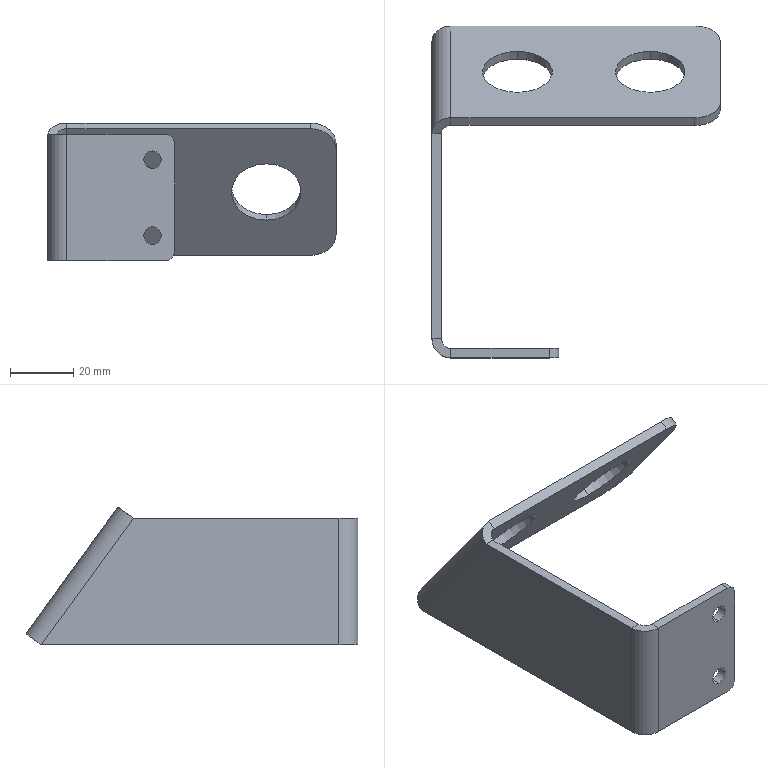Part | SolidWorks | features Fillet 2, ICE 2, EdgeFlange 1, FlatPattern 1, HoleWzd 1, SMBaseFlange 1, SheetMetal 1 | 1 solid | 34 faces | box 91 x 104.854 x 43.527 mm | volume 25604 mm3 | plane 18 | cylinder 16 | commonest cylinder face diameters 5.5 x4 6 x4 22 x4 12 x2 16 x2
STEP:
#1=CARTESIAN_POINT('',(-7.,3.,34.75));
#2=VERTEX_POINT('',#1);
#3=CARTESIAN_POINT('',(-7.,3.,29.25));
#4=VERTEX_POINT('',#3);
#5=CARTESIAN_POINT('',(-7.,3.,32.));
#6=DIRECTION('',(0.,-1.,0.));
#7=DIRECTION('',(1.,0.,0.));
#8=AXIS2_PLACEMENT_3D('',#5,#6,#7);
#9=CIRCLE('',#8,2.75);
#10=EDGE_CURVE('',#2,#4,#9,.T.);
#11=ORIENTED_EDGE('',*,*,#10,.F.);
#12=CARTESIAN_POINT('',(-7.,0.,34.75));
#13=VERTEX_POINT('',#12);
#14=CARTESIAN_POINT('',(-7.,0.,34.75));
#15=DIRECTION('',(0.,-1.,0.));
#16=VECTOR('',#15,1000.);
#17=LINE('',#14,#16);
#18=EDGE_CURVE('',#2,#13,#17,.T.);
#19=ORIENTED_EDGE('',*,*,#18,.T.);
#20=CARTESIAN_POINT('',(-7.,0.,29.25));
#21=VERTEX_POINT('',#20);
#22=CARTESIAN_POINT('',(-7.,0.,32.));
#23=DIRECTION('',(0.,-1.,0.));
#24=DIRECTION('',(0.,0.,-1.));
#25=AXIS2_PLACEMENT_3D('',#22,#23,#24);
#26=CIRCLE('',#25,2.75);
#27=EDGE_CURVE('',#13,#21,#26,.T.);
#28=ORIENTED_EDGE('',*,*,#27,.T.);
#29=CARTESIAN_POINT('',(-7.,0.,29.25));
#30=DIRECTION('',(0.,-1.,0.));
#31=VECTOR('',#30,1000.);
#32=LINE('',#29,#31);
#33=EDGE_CURVE('',#4,#21,#32,.T.);
#34=ORIENTED_EDGE('',*,*,#33,.F.);
#35=EDGE_LOOP('',(#11,#19,#28,#34));
#36=FACE_OUTER_BOUND('',#35,.T.);
#37=CARTESIAN_POINT('',(-7.,0.,32.));
#38=DIRECTION('',(0.,-1.,0.));
#39=DIRECTION('',(0.,0.,-1.));
#40=AXIS2_PLACEMENT_3D('',#37,#38,#39);
#41=CYLINDRICAL_SURFACE('',#40,2.75);
#42=ADVANCED_FACE('',(#36),#41,.F.);
#43=CARTESIAN_POINT('',(-7.,3.,10.75));
#44=VERTEX_POINT('',#43);
#45=CARTESIAN_POINT('',(-7.,3.,5.25));
#46=VERTEX_POINT('',#45);
#47=CARTESIAN_POINT('',(-7.,3.,8.));
#48=DIRECTION('',(0.,-1.,0.));
#49=DIRECTION('',(1.,0.,0.));
#50=AXIS2_PLACEMENT_3D('',#47,#48,#49);
#51=CIRCLE('',#50,2.75);
#52=EDGE_CURVE('',#44,#46,#51,.T.);
#53=ORIENTED_EDGE('',*,*,#52,.F.);
#54=CARTESIAN_POINT('',(-7.,0.,10.75));
#55=VERTEX_POINT('',#54);
#56=CARTESIAN_POINT('',(-7.,0.,10.75));
#57=DIRECTION('',(0.,-1.,0.));
#58=VECTOR('',#57,1000.);
#59=LINE('',#56,#58);
#60=EDGE_CURVE('',#44,#55,#59,.T.);
#61=ORIENTED_EDGE('',*,*,#60,.T.);
#62=CARTESIAN_POINT('',(-7.,0.,5.25));
#63=VERTEX_POINT('',#62);
#64=CARTESIAN_POINT('',(-7.,0.,8.));
#65=DIRECTION('',(0.,-1.,0.));
#66=DIRECTION('',(0.,0.,-1.));
#67=AXIS2_PLACEMENT_3D('',#64,#65,#66);
#68=CIRCLE('',#67,2.75);
#69=EDGE_CURVE('',#55,#63,#68,.T.);
#70=ORIENTED_EDGE('',*,*,#69,.T.);
#71=CARTESIAN_POINT('',(-7.,0.,5.25));
#72=DIRECTION('',(0.,-1.,0.));
#73=VECTOR('',#72,1000.);
#74=LINE('',#71,#73);
#75=EDGE_CURVE('',#46,#63,#74,.T.);
#76=ORIENTED_EDGE('',*,*,#75,.F.);
#77=EDGE_LOOP('',(#53,#61,#70,#76));
#78=FACE_OUTER_BOUND('',#77,.T.);
#79=CARTESIAN_POINT('',(-7.,0.,8.));
#80=DIRECTION('',(0.,-1.,0.));
#81=DIRECTION('',(0.,0.,-1.));
#82=AXIS2_PLACEMENT_3D('',#79,#80,#81);
#83=CYLINDRICAL_SURFACE('',#82,2.75);
#84=ADVANCED_FACE('',(#78),#83,.F.);
#85=CARTESIAN_POINT('',(-13.,94.362,12.864));
#86=VERTEX_POINT('',#85);
#87=CARTESIAN_POINT('',(-13.,81.431,30.663));
#88=VERTEX_POINT('',#87);
#89=CARTESIAN_POINT('',(-13.,87.896,21.763));
#90=DIRECTION('',(0.,0.809,0.5878));
#91=DIRECTION('',(0.,0.5878,-0.809));
#92=AXIS2_PLACEMENT_3D('',#89,#90,#91);
#93=CIRCLE('',#92,11.);
#94=EDGE_CURVE('',#86,#88,#93,.T.);
#95=ORIENTED_EDGE('',*,*,#94,.F.);
#96=CARTESIAN_POINT('',(-13.,96.789,14.628));
#97=VERTEX_POINT('',#96);
#98=CARTESIAN_POINT('',(-13.,26.483,-36.453));
#99=DIRECTION('',(0.,0.809,0.5878));
#100=VECTOR('',#99,1000.);
#101=LINE('',#98,#100);
#102=EDGE_CURVE('',#86,#97,#101,.T.);
#103=ORIENTED_EDGE('',*,*,#102,.T.);
#104=CARTESIAN_POINT('',(-13.,83.858,32.426));
#105=VERTEX_POINT('',#104);
#106=CARTESIAN_POINT('',(-13.,90.323,23.527));
#107=DIRECTION('',(0.,0.809,0.5878));
#108=DIRECTION('',(0.,-0.5878,0.809));
#109=AXIS2_PLACEMENT_3D('',#106,#107,#108);
#110=CIRCLE('',#109,11.);
#111=EDGE_CURVE('',#97,#105,#110,.T.);
#112=ORIENTED_EDGE('',*,*,#111,.T.);
#113=CARTESIAN_POINT('',(-13.,13.552,-18.654));
#114=DIRECTION('',(0.,0.809,0.5878));
#115=VECTOR('',#114,1000.);
#116=LINE('',#113,#115);
#117=EDGE_CURVE('',#88,#105,#116,.T.);
#118=ORIENTED_EDGE('',*,*,#117,.F.);
#119=EDGE_LOOP('',(#95,#103,#112,#118));
#120=FACE_OUTER_BOUND('',#119,.T.);
#121=CARTESIAN_POINT('',(-13.,20.017,-27.554));
#122=DIRECTION('',(0.,0.809,0.5878));
#123=DIRECTION('',(0.,-0.5878,0.809));
#124=AXIS2_PLACEMENT_3D('',#121,#122,#123);
#125=CYLINDRICAL_SURFACE('',#124,11.);
#126=ADVANCED_FACE('',(#120),#125,.F.);
#127=CARTESIAN_POINT('',(29.,94.362,12.864));
#128=VERTEX_POINT('',#127);
#129=CARTESIAN_POINT('',(29.,81.431,30.663));
#130=VERTEX_POINT('',#129);
#131=CARTESIAN_POINT('',(29.,87.896,21.763));
#132=DIRECTION('',(0.,0.809,0.5878));
#133=DIRECTION('',(0.,0.5878,-0.809));
#134=AXIS2_PLACEMENT_3D('',#131,#132,#133);
#135=CIRCLE('',#134,11.);
#136=EDGE_CURVE('',#128,#130,#135,.T.);
#137=ORIENTED_EDGE('',*,*,#136,.F.);
#138=CARTESIAN_POINT('',(29.,96.789,14.628));
#139=VERTEX_POINT('',#138);
#140=CARTESIAN_POINT('',(29.,26.483,-36.453));
#141=DIRECTION('',(0.,0.809,0.5878));
#142=VECTOR('',#141,1000.);
#143=LINE('',#140,#142);
#144=EDGE_CURVE('',#128,#139,#143,.T.);
#145=ORIENTED_EDGE('',*,*,#144,.T.);
#146=CARTESIAN_POINT('',(29.,83.858,32.426));
#147=VERTEX_POINT('',#146);
#148=CARTESIAN_POINT('',(29.,90.323,23.527));
#149=DIRECTION('',(0.,0.809,0.5878));
#150=DIRECTION('',(0.,-0.5878,0.809));
#151=AXIS2_PLACEMENT_3D('',#148,#149,#150);
#152=CIRCLE('',#151,11.);
#153=EDGE_CURVE('',#139,#147,#152,.T.);
#154=ORIENTED_EDGE('',*,*,#153,.T.);
#155=CARTESIAN_POINT('',(29.,13.552,-18.654));
#156=DIRECTION('',(0.,0.809,0.5878));
#157=VECTOR('',#156,1000.);
#158=LINE('',#155,#157);
#159=EDGE_CURVE('',#130,#147,#158,.T.);
#160=ORIENTED_EDGE('',*,*,#159,.F.);
#161=EDGE_LOOP('',(#137,#145,#154,#160));
#162=FACE_OUTER_BOUND('',#161,.T.);
#163=CARTESIAN_POINT('',(29.,20.017,-27.554));
#164=DIRECTION('',(0.,0.809,0.5878));
#165=DIRECTION('',(0.,-0.5878,0.809));
#166=AXIS2_PLACEMENT_3D('',#163,#164,#165);
#167=CYLINDRICAL_SURFACE('',#166,11.);
#168=ADVANCED_FACE('',(#162),#167,.F.);
#169=CARTESIAN_POINT('',(-37.,6.,40.));
#170=VERTEX_POINT('',#169);
#171=CARTESIAN_POINT('',(-37.,70.938,40.));
#172=VERTEX_POINT('',#171);
#173=CARTESIAN_POINT('',(-37.,0.,40.));
#174=DIRECTION('',(0.,1.,0.));
#175=VECTOR('',#174,1000.);
#176=LINE('',#173,#175);
#177=EDGE_CURVE('',#170,#172,#176,.T.);
#178=ORIENTED_EDGE('',*,*,#177,.T.);
#179=CARTESIAN_POINT('',(-40.,70.938,40.));
#180=VERTEX_POINT('',#179);
#181=CARTESIAN_POINT('',(-37.,70.938,40.));
#182=DIRECTION('',(-1.,0.,0.));
#183=VECTOR('',#182,1000.);
#184=LINE('',#181,#183);
#185=EDGE_CURVE('',#172,#180,#184,.T.);
#186=ORIENTED_EDGE('',*,*,#185,.T.);
#187=CARTESIAN_POINT('',(-40.,6.,40.));
#188=VERTEX_POINT('',#187);
#189=CARTESIAN_POINT('',(-40.,0.,40.));
#190=DIRECTION('',(0.,1.,0.));
#191=VECTOR('',#190,1000.);
#192=LINE('',#189,#191);
#193=EDGE_CURVE('',#188,#180,#192,.T.);
#194=ORIENTED_EDGE('',*,*,#193,.F.);
#195=CARTESIAN_POINT('',(-40.,6.,40.));
#196=DIRECTION('',(1.,0.,0.));
#197=VECTOR('',#196,1000.);
#198=LINE('',#195,#197);
#199=EDGE_CURVE('',#188,#170,#198,.T.);
#200=ORIENTED_EDGE('',*,*,#199,.T.);
#201=EDGE_LOOP('',(#178,#186,#194,#200));
#202=FACE_OUTER_BOUND('',#201,.T.);
#203=CARTESIAN_POINT('',(-34.,3.,40.));
#204=DIRECTION('',(0.,0.,1.));
#205=DIRECTION('',(1.,0.,0.));
#206=AXIS2_PLACEMENT_3D('',#203,#204,#205);
#207=PLANE('',#206);
#208=ADVANCED_FACE('',(#202),#207,.T.);
#209=CARTESIAN_POINT('',(-37.,100.,0.));
#210=VERTEX_POINT('',#209);
#211=CARTESIAN_POINT('',(-37.,46.43,73.733));
#212=DIRECTION('',(0.,-0.5878,0.809));
#213=VECTOR('',#212,1000.);
#214=LINE('',#211,#213);
#215=EDGE_CURVE('',#210,#172,#214,.T.);
#216=ORIENTED_EDGE('',*,*,#215,.T.);
#217=ORIENTED_EDGE('',*,*,#177,.F.);
#218=CARTESIAN_POINT('',(-37.,6.,0.));
#219=VERTEX_POINT('',#218);
#220=CARTESIAN_POINT('',(-37.,6.,40.));
#221=DIRECTION('',(0.,0.,-1.));
#222=VECTOR('',#221,1000.);
#223=LINE('',#220,#222);
#224=EDGE_CURVE('',#170,#219,#223,.T.);
#225=ORIENTED_EDGE('',*,*,#224,.T.);
#226=CARTESIAN_POINT('',(-37.,0.,0.));
#227=DIRECTION('',(0.,1.,0.));
#228=VECTOR('',#227,1000.);
#229=LINE('',#226,#228);
#230=EDGE_CURVE('',#219,#210,#229,.T.);
#231=ORIENTED_EDGE('',*,*,#230,.T.);
#232=EDGE_LOOP('',(#216,#217,#225,#231));
#233=FACE_OUTER_BOUND('',#232,.T.);
#234=CARTESIAN_POINT('',(-37.,0.,40.));
#235=DIRECTION('',(-1.,0.,0.));
#236=DIRECTION('',(0.,0.,1.));
#237=AXIS2_PLACEMENT_3D('',#234,#235,#236);
#238=PLANE('',#237);
#239=ADVANCED_FACE('',(#233),#238,.F.);
#240=ORIENTED_EDGE('',*,*,#193,.T.);
#241=CARTESIAN_POINT('',(-40.,100.,0.));
#242=VERTEX_POINT('',#241);
#243=CARTESIAN_POINT('',(-40.,46.43,73.733));
#244=DIRECTION('',(0.,-0.5878,0.809));
#245=VECTOR('',#244,1000.);
#246=LINE('',#243,#245);
#247=EDGE_CURVE('',#242,#180,#246,.T.);
#248=ORIENTED_EDGE('',*,*,#247,.F.);
#249=CARTESIAN_POINT('',(-40.,6.,0.));
#250=VERTEX_POINT('',#249);
#251=CARTESIAN_POINT('',(-40.,0.,0.));
#252=DIRECTION('',(0.,1.,0.));
#253=VECTOR('',#252,1000.);
#254=LINE('',#251,#253);
#255=EDGE_CURVE('',#250,#242,#254,.T.);
#256=ORIENTED_EDGE('',*,*,#255,.F.);
#257=CARTESIAN_POINT('',(-40.,6.,40.));
#258=DIRECTION('',(0.,0.,-1.));
#259=VECTOR('',#258,1000.);
#260=LINE('',#257,#259);
#261=EDGE_CURVE('',#188,#250,#260,.T.);
#262=ORIENTED_EDGE('',*,*,#261,.F.);
#263=EDGE_LOOP('',(#240,#248,#256,#262));
#264=FACE_OUTER_BOUND('',#263,.T.);
#265=CARTESIAN_POINT('',(-40.,0.,40.));
#266=DIRECTION('',(-1.,0.,0.));
#267=DIRECTION('',(0.,0.,1.));
#268=AXIS2_PLACEMENT_3D('',#265,#266,#267);
#269=PLANE('',#268);
#270=ADVANCED_FACE('',(#264),#269,.T.);
#271=ORIENTED_EDGE('',*,*,#199,.F.);
#272=CARTESIAN_POINT('',(-34.,0.,40.));
#273=VERTEX_POINT('',#272);
#274=CARTESIAN_POINT('',(-34.,6.,40.));
#275=DIRECTION('',(0.,0.,-1.));
#276=DIRECTION('',(1.,0.,0.));
#277=AXIS2_PLACEMENT_3D('',#274,#275,#276);
#278=CIRCLE('',#277,6.);
#279=EDGE_CURVE('',#273,#188,#278,.T.);
#280=ORIENTED_EDGE('',*,*,#279,.F.);
#281=CARTESIAN_POINT('',(-34.,3.,40.));
#282=VERTEX_POINT('',#281);
#283=CARTESIAN_POINT('',(-34.,3.,40.));
#284=DIRECTION('',(0.,-1.,0.));
#285=VECTOR('',#284,1000.);
#286=LINE('',#283,#285);
#287=EDGE_CURVE('',#282,#273,#286,.T.);
#288=ORIENTED_EDGE('',*,*,#287,.F.);
#289=CARTESIAN_POINT('',(-34.,6.,40.));
#290=DIRECTION('',(0.,0.,-1.));
#291=DIRECTION('',(1.,0.,0.));
#292=AXIS2_PLACEMENT_3D('',#289,#290,#291);
#293=CIRCLE('',#292,3.);
#294=EDGE_CURVE('',#282,#170,#293,.T.);
#295=ORIENTED_EDGE('',*,*,#294,.T.);
#296=EDGE_LOOP('',(#271,#280,#288,#295));
#297=FACE_OUTER_BOUND('',#296,.T.);
#298=CARTESIAN_POINT('',(-40.,6.,40.));
#299=DIRECTION('',(0.,0.,1.));
#300=DIRECTION('',(1.,0.,0.));
#301=AXIS2_PLACEMENT_3D('',#298,#299,#300);
#302=PLANE('',#301);
#303=ADVANCED_FACE('',(#297),#302,.T.);
#304=CARTESIAN_POINT('',(-34.,0.,0.));
#305=VERTEX_POINT('',#304);
#306=CARTESIAN_POINT('',(-34.,3.,0.));
#307=VERTEX_POINT('',#306);
#308=CARTESIAN_POINT('',(-34.,0.,0.));
#309=DIRECTION('',(0.,1.,0.));
#310=VECTOR('',#309,1000.);
#311=LINE('',#308,#310);
#312=EDGE_CURVE('',#305,#307,#311,.T.);
#313=ORIENTED_EDGE('',*,*,#312,.F.);
#314=CARTESIAN_POINT('',(-34.,6.,0.));
#315=DIRECTION('',(0.,0.,-1.));
#316=DIRECTION('',(1.,0.,0.));
#317=AXIS2_PLACEMENT_3D('',#314,#315,#316);
#318=CIRCLE('',#317,6.);
#319=EDGE_CURVE('',#305,#250,#318,.T.);
#320=ORIENTED_EDGE('',*,*,#319,.T.);
#321=CARTESIAN_POINT('',(-37.,6.,0.));
#322=DIRECTION('',(-1.,0.,0.));
#323=VECTOR('',#322,1000.);
#324=LINE('',#321,#323);
#325=EDGE_CURVE('',#219,#250,#324,.T.);
#326=ORIENTED_EDGE('',*,*,#325,.F.);
#327=CARTESIAN_POINT('',(-34.,6.,0.));
#328=DIRECTION('',(0.,0.,-1.));
#329=DIRECTION('',(1.,0.,0.));
#330=AXIS2_PLACEMENT_3D('',#327,#328,#329);
#331=CIRCLE('',#330,3.);
#332=EDGE_CURVE('',#307,#219,#331,.T.);
#333=ORIENTED_EDGE('',*,*,#332,.F.);
#334=EDGE_LOOP('',(#313,#320,#326,#333));
#335=FACE_OUTER_BOUND('',#334,.T.);
#336=CARTESIAN_POINT('',(-34.,0.,0.));
#337=DIRECTION('',(0.,0.,-1.));
#338=DIRECTION('',(-1.,0.,0.));
#339=AXIS2_PLACEMENT_3D('',#336,#337,#338);
#340=PLANE('',#339);
#341=ADVANCED_FACE('',(#335),#340,.T.);
#342=CARTESIAN_POINT('',(-3.,3.,0.));
#343=VERTEX_POINT('',#342);
#344=CARTESIAN_POINT('',(0.,3.,0.));
#345=DIRECTION('',(-1.,0.,0.));
#346=VECTOR('',#345,1000.);
#347=LINE('',#344,#346);
#348=EDGE_CURVE('',#343,#307,#347,.T.);
#349=ORIENTED_EDGE('',*,*,#348,.F.);
#350=CARTESIAN_POINT('',(-3.,0.,0.));
#351=VERTEX_POINT('',#350);
#352=CARTESIAN_POINT('',(-3.,6.,0.));
#353=DIRECTION('',(0.,-1.,0.));
#354=VECTOR('',#353,1000.);
#355=LINE('',#352,#354);
#356=EDGE_CURVE('',#343,#351,#355,.T.);
#357=ORIENTED_EDGE('',*,*,#356,.T.);
#358=CARTESIAN_POINT('',(0.,0.,0.));
#359=DIRECTION('',(-1.,0.,0.));
#360=VECTOR('',#359,1000.);
#361=LINE('',#358,#360);
#362=EDGE_CURVE('',#351,#305,#361,.T.);
#363=ORIENTED_EDGE('',*,*,#362,.T.);
#364=ORIENTED_EDGE('',*,*,#312,.T.);
#365=EDGE_LOOP('',(#349,#357,#363,#364));
#366=FACE_OUTER_BOUND('',#365,.T.);
#367=CARTESIAN_POINT('',(-37.,6.,0.));
#368=DIRECTION('',(0.,0.,-1.));
#369=DIRECTION('',(-1.,0.,0.));
#370=AXIS2_PLACEMENT_3D('',#367,#368,#369);
#371=PLANE('',#370);
#372=ADVANCED_FACE('',(#366),#371,.T.);
#373=ORIENTED_EDGE('',*,*,#319,.F.);
#374=CARTESIAN_POINT('',(-34.,0.,40.));
#375=DIRECTION('',(0.,0.,-1.));
#376=VECTOR('',#375,1000.);
#377=LINE('',#374,#376);
#378=EDGE_CURVE('',#273,#305,#377,.T.);
#379=ORIENTED_EDGE('',*,*,#378,.F.);
#380=ORIENTED_EDGE('',*,*,#279,.T.);
#381=ORIENTED_EDGE('',*,*,#261,.T.);
#382=EDGE_LOOP('',(#373,#379,#380,#381));
#383=FACE_OUTER_BOUND('',#382,.T.);
#384=CARTESIAN_POINT('',(-34.,6.,40.));
#385=DIRECTION('',(0.,0.,-1.));
#386=DIRECTION('',(-1.,0.,0.));
#387=AXIS2_PLACEMENT_3D('',#384,#385,#386);
#388=CYLINDRICAL_SURFACE('',#387,6.);
#389=ADVANCED_FACE('',(#383),#388,.T.);
#390=CARTESIAN_POINT('',(-7.,0.,32.));
#391=DIRECTION('',(0.,-1.,0.));
#392=DIRECTION('',(0.,0.,-1.));
#393=AXIS2_PLACEMENT_3D('',#390,#391,#392);
#394=CIRCLE('',#393,2.75);
#395=EDGE_CURVE('',#21,#13,#394,.T.);
#396=ORIENTED_EDGE('',*,*,#395,.F.);
#397=ORIENTED_EDGE('',*,*,#27,.F.);
#398=EDGE_LOOP('',(#396,#397));
#399=FACE_BOUND('',#398,.T.);
#400=CARTESIAN_POINT('',(-7.,0.,8.));
#401=DIRECTION('',(0.,-1.,0.));
#402=DIRECTION('',(0.,0.,-1.));
#403=AXIS2_PLACEMENT_3D('',#400,#401,#402);
#404=CIRCLE('',#403,2.75);
#405=EDGE_CURVE('',#63,#55,#404,.T.);
#406=ORIENTED_EDGE('',*,*,#405,.F.);
#407=ORIENTED_EDGE('',*,*,#69,.F.);
#408=EDGE_LOOP('',(#406,#407));
#409=FACE_BOUND('',#408,.T.);
#410=ORIENTED_EDGE('',*,*,#362,.F.);
#411=CARTESIAN_POINT('',(0.,0.,3.));
#412=VERTEX_POINT('',#411);
#413=CARTESIAN_POINT('',(-3.,0.,3.));
#414=DIRECTION('',(0.,-1.,0.));
#415=DIRECTION('',(1.,0.,0.));
#416=AXIS2_PLACEMENT_3D('',#413,#414,#415);
#417=CIRCLE('',#416,3.);
#418=EDGE_CURVE('',#351,#412,#417,.T.);
#419=ORIENTED_EDGE('',*,*,#418,.T.);
#420=CARTESIAN_POINT('',(0.,0.,37.));
#421=VERTEX_POINT('',#420);
#422=CARTESIAN_POINT('',(0.,0.,40.));
#423=DIRECTION('',(0.,0.,-1.));
#424=VECTOR('',#423,1000.);
#425=LINE('',#422,#424);
#426=EDGE_CURVE('',#421,#412,#425,.T.);
#427=ORIENTED_EDGE('',*,*,#426,.F.);
#428=CARTESIAN_POINT('',(-3.,0.,40.));
#429=VERTEX_POINT('',#428);
#430=CARTESIAN_POINT('',(-3.,0.,37.));
#431=DIRECTION('',(0.,-1.,0.));
#432=DIRECTION('',(1.,0.,0.));
#433=AXIS2_PLACEMENT_3D('',#430,#431,#432);
#434=CIRCLE('',#433,3.);
#435=EDGE_CURVE('',#421,#429,#434,.T.);
#436=ORIENTED_EDGE('',*,*,#435,.T.);
#437=CARTESIAN_POINT('',(0.,0.,40.));
#438=DIRECTION('',(-1.,0.,0.));
#439=VECTOR('',#438,1000.);
#440=LINE('',#437,#439);
#441=EDGE_CURVE('',#429,#273,#440,.T.);
#442=ORIENTED_EDGE('',*,*,#441,.T.);
#443=ORIENTED_EDGE('',*,*,#378,.T.);
#444=EDGE_LOOP('',(#410,#419,#427,#436,#442,#443));
#445=FACE_OUTER_BOUND('',#444,.T.);
#446=CARTESIAN_POINT('',(0.,0.,40.));
#447=DIRECTION('',(0.,-1.,0.));
#448=DIRECTION('',(1.,0.,0.));
#449=AXIS2_PLACEMENT_3D('',#446,#447,#448);
#450=PLANE('',#449);
#451=ADVANCED_FACE('',(#399,#409,#445),#450,.T.);
#452=ORIENTED_EDGE('',*,*,#426,.T.);
#453=CARTESIAN_POINT('',(0.,3.,3.));
#454=VERTEX_POINT('',#453);
#455=CARTESIAN_POINT('',(0.,3.,3.));
#456=DIRECTION('',(0.,1.,0.));
#457=VECTOR('',#456,1000.);
#458=LINE('',#455,#457);
#459=EDGE_CURVE('',#412,#454,#458,.T.);
#460=ORIENTED_EDGE('',*,*,#459,.T.);
#461=CARTESIAN_POINT('',(0.,3.,37.));
#462=VERTEX_POINT('',#461);
#463=CARTESIAN_POINT('',(0.,3.,40.));
#464=DIRECTION('',(0.,0.,-1.));
#465=VECTOR('',#464,1000.);
#466=LINE('',#463,#465);
#467=EDGE_CURVE('',#462,#454,#466,.T.);
#468=ORIENTED_EDGE('',*,*,#467,.F.);
#469=CARTESIAN_POINT('',(0.,3.,37.));
#470=DIRECTION('',(0.,-1.,0.));
#471=VECTOR('',#470,1000.);
#472=LINE('',#469,#471);
#473=EDGE_CURVE('',#462,#421,#472,.T.);
#474=ORIENTED_EDGE('',*,*,#473,.T.);
#475=EDGE_LOOP('',(#452,#460,#468,#474));
#476=FACE_OUTER_BOUND('',#475,.T.);
#477=CARTESIAN_POINT('',(0.,3.,40.));
#478=DIRECTION('',(1.,0.,0.));
#479=DIRECTION('',(0.,1.,0.));
#480=AXIS2_PLACEMENT_3D('',#477,#478,#479);
#481=PLANE('',#480);
#482=ADVANCED_FACE('',(#476),#481,.T.);
#483=CARTESIAN_POINT('',(-7.,3.,32.));
#484=DIRECTION('',(0.,-1.,0.));
#485=DIRECTION('',(1.,0.,0.));
#486=AXIS2_PLACEMENT_3D('',#483,#484,#485);
#487=CIRCLE('',#486,2.75);
#488=EDGE_CURVE('',#4,#2,#487,.T.);
#489=ORIENTED_EDGE('',*,*,#488,.T.);
#490=ORIENTED_EDGE('',*,*,#10,.T.);
#491=EDGE_LOOP('',(#489,#490));
#492=FACE_BOUND('',#491,.T.);
#493=CARTESIAN_POINT('',(-7.,3.,8.));
#494=DIRECTION('',(0.,-1.,0.));
#495=DIRECTION('',(1.,0.,0.));
#496=AXIS2_PLACEMENT_3D('',#493,#494,#495);
#497=CIRCLE('',#496,2.75);
#498=EDGE_CURVE('',#46,#44,#497,.T.);
#499=ORIENTED_EDGE('',*,*,#498,.T.);
#500=ORIENTED_EDGE('',*,*,#52,.T.);
#501=EDGE_LOOP('',(#499,#500));
#502=FACE_BOUND('',#501,.T.);
#503=ORIENTED_EDGE('',*,*,#467,.T.);
#504=CARTESIAN_POINT('',(-3.,3.,3.));
#505=DIRECTION('',(0.,1.,0.));
#506=DIRECTION('',(1.,0.,0.));
#507=AXIS2_PLACEMENT_3D('',#504,#505,#506);
#508=CIRCLE('',#507,3.);
#509=EDGE_CURVE('',#454,#343,#508,.T.);
#510=ORIENTED_EDGE('',*,*,#509,.T.);
#511=ORIENTED_EDGE('',*,*,#348,.T.);
#512=CARTESIAN_POINT('',(-34.,3.,40.));
#513=DIRECTION('',(0.,0.,-1.));
#514=VECTOR('',#513,1000.);
#515=LINE('',#512,#514);
#516=EDGE_CURVE('',#282,#307,#515,.T.);
#517=ORIENTED_EDGE('',*,*,#516,.F.);
#518=CARTESIAN_POINT('',(-3.,3.,40.));
#519=VERTEX_POINT('',#518);
#520=CARTESIAN_POINT('',(0.,3.,40.));
#521=DIRECTION('',(-1.,0.,0.));
#522=VECTOR('',#521,1000.);
#523=LINE('',#520,#522);
#524=EDGE_CURVE('',#519,#282,#523,.T.);
#525=ORIENTED_EDGE('',*,*,#524,.F.);
#526=CARTESIAN_POINT('',(-3.,3.,37.));
#527=DIRECTION('',(0.,1.,0.));
#528=DIRECTION('',(1.,0.,0.));
#529=AXIS2_PLACEMENT_3D('',#526,#527,#528);
#530=CIRCLE('',#529,3.);
#531=EDGE_CURVE('',#519,#462,#530,.T.);
#532=ORIENTED_EDGE('',*,*,#531,.T.);
#533=EDGE_LOOP('',(#503,#510,#511,#517,#525,#532));
#534=FACE_OUTER_BOUND('',#533,.T.);
#535=CARTESIAN_POINT('',(0.,3.,40.));
#536=DIRECTION('',(0.,-1.,0.));
#537=DIRECTION('',(1.,0.,0.));
#538=AXIS2_PLACEMENT_3D('',#535,#536,#537);
#539=PLANE('',#538);
#540=ADVANCED_FACE('',(#492,#502,#534),#539,.F.);
#541=ORIENTED_EDGE('',*,*,#332,.T.);
#542=ORIENTED_EDGE('',*,*,#224,.F.);
#543=ORIENTED_EDGE('',*,*,#294,.F.);
#544=ORIENTED_EDGE('',*,*,#516,.T.);
#545=EDGE_LOOP('',(#541,#542,#543,#544));
#546=FACE_OUTER_BOUND('',#545,.T.);
#547=CARTESIAN_POINT('',(-34.,6.,40.));
#548=DIRECTION('',(0.,0.,-1.));
#549=DIRECTION('',(-1.,0.,0.));
#550=AXIS2_PLACEMENT_3D('',#547,#548,#549);
#551=CYLINDRICAL_SURFACE('',#550,3.);
#552=ADVANCED_FACE('',(#546),#551,.F.);
#553=ORIENTED_EDGE('',*,*,#441,.F.);
#554=CARTESIAN_POINT('',(-3.,6.,40.));
#555=DIRECTION('',(0.,1.,0.));
#556=VECTOR('',#555,1000.);
#557=LINE('',#554,#556);
#558=EDGE_CURVE('',#429,#519,#557,.T.);
#559=ORIENTED_EDGE('',*,*,#558,.T.);
#560=ORIENTED_EDGE('',*,*,#524,.T.);
#561=ORIENTED_EDGE('',*,*,#287,.T.);
#562=EDGE_LOOP('',(#553,#559,#560,#561));
#563=FACE_OUTER_BOUND('',#562,.T.);
#564=CARTESIAN_POINT('',(-34.,6.,40.));
#565=DIRECTION('',(0.,0.,1.));
#566=DIRECTION('',(1.,0.,0.));
#567=AXIS2_PLACEMENT_3D('',#564,#565,#566);
#568=PLANE('',#567);
#569=ADVANCED_FACE('',(#563),#568,.T.);
#570=ORIENTED_EDGE('',*,*,#230,.F.);
#571=ORIENTED_EDGE('',*,*,#325,.T.);
#572=ORIENTED_EDGE('',*,*,#255,.T.);
#573=CARTESIAN_POINT('',(-40.,100.,0.));
#574=DIRECTION('',(1.,0.,0.));
#575=VECTOR('',#574,1000.);
#576=LINE('',#573,#575);
#577=EDGE_CURVE('',#242,#210,#576,.T.);
#578=ORIENTED_EDGE('',*,*,#577,.T.);
#579=EDGE_LOOP('',(#570,#571,#572,#578));
#580=FACE_OUTER_BOUND('',#579,.T.);
#581=CARTESIAN_POINT('',(-34.,6.,0.));
#582=DIRECTION('',(0.,0.,1.));
#583=DIRECTION('',(1.,0.,0.));
#584=AXIS2_PLACEMENT_3D('',#581,#582,#583);
#585=PLANE('',#584);
#586=ADVANCED_FACE('',(#580),#585,.F.);
#587=CARTESIAN_POINT('',(-34.,102.427,1.763));
#588=VERTEX_POINT('',#587);
#589=CARTESIAN_POINT('',(-34.,104.854,3.527));
#590=VERTEX_POINT('',#589);
#591=CARTESIAN_POINT('',(-34.,104.854,3.527));
#592=DIRECTION('',(0.,0.809,0.5878));
#593=VECTOR('',#592,1000.);
#594=LINE('',#591,#593);
#595=EDGE_CURVE('',#588,#590,#594,.T.);
#596=ORIENTED_EDGE('',*,*,#595,.F.);
#597=CARTESIAN_POINT('',(-34.,100.,0.));
#598=DIRECTION('',(0.,0.5878,-0.809));
#599=DIRECTION('',(0.,-0.809,-0.5878));
#600=AXIS2_PLACEMENT_3D('',#597,#598,#599);
#601=CIRCLE('',#600,3.);
#602=EDGE_CURVE('',#210,#588,#601,.T.);
#603=ORIENTED_EDGE('',*,*,#602,.F.);
#604=ORIENTED_EDGE('',*,*,#577,.F.);
#605=CARTESIAN_POINT('',(-34.,100.,0.));
#606=DIRECTION('',(0.,0.5878,-0.809));
#607=DIRECTION('',(0.,-0.809,-0.5878));
#608=AXIS2_PLACEMENT_3D('',#605,#606,#607);
#609=CIRCLE('',#608,6.);
#610=EDGE_CURVE('',#242,#590,#609,.T.);
#611=ORIENTED_EDGE('',*,*,#610,.T.);
#612=EDGE_LOOP('',(#596,#603,#604,#611));
#613=FACE_OUTER_BOUND('',#612,.T.);
#614=CARTESIAN_POINT('',(-34.,100.,0.));
#615=DIRECTION('',(0.,0.5878,-0.809));
#616=DIRECTION('',(0.,0.809,0.5878));
#617=AXIS2_PLACEMENT_3D('',#614,#615,#616);
#618=PLANE('',#617);
#619=ADVANCED_FACE('',(#613),#618,.T.);
#620=CARTESIAN_POINT('',(-34.,73.365,41.763));
#621=VERTEX_POINT('',#620);
#622=CARTESIAN_POINT('',(-34.,70.938,40.));
#623=DIRECTION('',(0.,-0.5878,0.809));
#624=DIRECTION('',(0.,-0.809,-0.5878));
#625=AXIS2_PLACEMENT_3D('',#622,#623,#624);
#626=CIRCLE('',#625,3.);
#627=EDGE_CURVE('',#621,#172,#626,.T.);
#628=ORIENTED_EDGE('',*,*,#627,.F.);
#629=CARTESIAN_POINT('',(-34.,75.792,43.527));
#630=VERTEX_POINT('',#629);
#631=CARTESIAN_POINT('',(-34.,73.365,41.763));
#632=DIRECTION('',(0.,0.809,0.5878));
#633=VECTOR('',#632,1000.);
#634=LINE('',#631,#633);
#635=EDGE_CURVE('',#621,#630,#634,.T.);
#636=ORIENTED_EDGE('',*,*,#635,.T.);
#637=CARTESIAN_POINT('',(-34.,70.938,40.));
#638=DIRECTION('',(0.,-0.5878,0.809));
#639=DIRECTION('',(0.,-0.809,-0.5878));
#640=AXIS2_PLACEMENT_3D('',#637,#638,#639);
#641=CIRCLE('',#640,6.);
#642=EDGE_CURVE('',#630,#180,#641,.T.);
#643=ORIENTED_EDGE('',*,*,#642,.T.);
#644=ORIENTED_EDGE('',*,*,#185,.F.);
#645=EDGE_LOOP('',(#628,#636,#643,#644));
#646=FACE_OUTER_BOUND('',#645,.T.);
#647=CARTESIAN_POINT('',(-34.,70.938,40.));
#648=DIRECTION('',(0.,0.5878,-0.809));
#649=DIRECTION('',(0.,0.809,0.5878));
#650=AXIS2_PLACEMENT_3D('',#647,#648,#649);
#651=PLANE('',#650);
#652=ADVANCED_FACE('',(#646),#651,.F.);
#653=ORIENTED_EDGE('',*,*,#247,.T.);
#654=ORIENTED_EDGE('',*,*,#642,.F.);
#655=CARTESIAN_POINT('',(-34.,104.854,3.527));
#656=DIRECTION('',(0.,0.5878,-0.809));
#657=VECTOR('',#656,1000.);
#658=LINE('',#655,#657);
#659=EDGE_CURVE('',#630,#590,#658,.T.);
#660=ORIENTED_EDGE('',*,*,#659,.T.);
#661=ORIENTED_EDGE('',*,*,#610,.F.);
#662=EDGE_LOOP('',(#653,#654,#660,#661));
#663=FACE_OUTER_BOUND('',#662,.T.);
#664=CARTESIAN_POINT('',(-34.,70.938,40.));
#665=DIRECTION('',(0.,-0.5878,0.809));
#666=DIRECTION('',(0.,0.809,0.5878));
#667=AXIS2_PLACEMENT_3D('',#664,#665,#666);
#668=CYLINDRICAL_SURFACE('',#667,6.);
#669=ADVANCED_FACE('',(#663),#668,.T.);
#670=ORIENTED_EDGE('',*,*,#215,.F.);
#671=ORIENTED_EDGE('',*,*,#602,.T.);
#672=CARTESIAN_POINT('',(-34.,102.427,1.763));
#673=DIRECTION('',(0.,-0.5878,0.809));
#674=VECTOR('',#673,1000.);
#675=LINE('',#672,#674);
#676=EDGE_CURVE('',#588,#621,#675,.T.);
#677=ORIENTED_EDGE('',*,*,#676,.T.);
#678=ORIENTED_EDGE('',*,*,#627,.T.);
#679=EDGE_LOOP('',(#670,#671,#677,#678));
#680=FACE_OUTER_BOUND('',#679,.T.);
#681=CARTESIAN_POINT('',(-34.,70.938,40.));
#682=DIRECTION('',(0.,-0.5878,0.809));
#683=DIRECTION('',(0.,0.809,0.5878));
#684=AXIS2_PLACEMENT_3D('',#681,#682,#683);
#685=CYLINDRICAL_SURFACE('',#684,3.);
#686=ADVANCED_FACE('',(#680),#685,.F.);
#687=CARTESIAN_POINT('',(43.,104.854,3.527));
#688=VERTEX_POINT('',#687);
#689=CARTESIAN_POINT('',(0.,104.854,3.527));
#690=DIRECTION('',(-1.,0.,0.));
#691=VECTOR('',#690,1000.);
#692=LINE('',#689,#691);
#693=EDGE_CURVE('',#688,#590,#692,.T.);
#694=ORIENTED_EDGE('',*,*,#693,.F.);
#695=CARTESIAN_POINT('',(43.,102.427,1.763));
#696=VERTEX_POINT('',#695);
#697=CARTESIAN_POINT('',(43.,104.854,3.527));
#698=DIRECTION('',(0.,-0.809,-0.5878));
#699=VECTOR('',#698,1000.);
#700=LINE('',#697,#699);
#701=EDGE_CURVE('',#688,#696,#700,.T.);
#702=ORIENTED_EDGE('',*,*,#701,.T.);
#703=CARTESIAN_POINT('',(-37.,102.427,1.763));
#704=DIRECTION('',(-1.,0.,0.));
#705=VECTOR('',#704,1000.);
#706=LINE('',#703,#705);
#707=EDGE_CURVE('',#696,#588,#706,.T.);
#708=ORIENTED_EDGE('',*,*,#707,.T.);
#709=ORIENTED_EDGE('',*,*,#595,.T.);
#710=EDGE_LOOP('',(#694,#702,#708,#709));
#711=FACE_OUTER_BOUND('',#710,.T.);
#712=CARTESIAN_POINT('',(-37.,104.854,3.527));
#713=DIRECTION('',(0.,-0.5878,0.809));
#714=DIRECTION('',(0.,-0.809,-0.5878));
#715=AXIS2_PLACEMENT_3D('',#712,#713,#714);
#716=PLANE('',#715);
#717=ADVANCED_FACE('',(#711),#716,.F.);
#718=CARTESIAN_POINT('',(43.,73.365,41.763));
#719=VERTEX_POINT('',#718);
#720=CARTESIAN_POINT('',(51.,73.365,41.763));
#721=DIRECTION('',(1.,0.,0.));
#722=VECTOR('',#721,1000.);
#723=LINE('',#720,#722);
#724=EDGE_CURVE('',#621,#719,#723,.T.);
#725=ORIENTED_EDGE('',*,*,#724,.T.);
#726=CARTESIAN_POINT('',(43.,75.792,43.527));
#727=VERTEX_POINT('',#726);
#728=CARTESIAN_POINT('',(43.,75.792,43.527));
#729=DIRECTION('',(0.,0.809,0.5878));
#730=VECTOR('',#729,1000.);
#731=LINE('',#728,#730);
#732=EDGE_CURVE('',#719,#727,#731,.T.);
#733=ORIENTED_EDGE('',*,*,#732,.T.);
#734=CARTESIAN_POINT('',(0.,75.792,43.527));
#735=DIRECTION('',(1.,0.,0.));
#736=VECTOR('',#735,1000.);
#737=LINE('',#734,#736);
#738=EDGE_CURVE('',#630,#727,#737,.T.);
#739=ORIENTED_EDGE('',*,*,#738,.F.);
#740=ORIENTED_EDGE('',*,*,#635,.F.);
#741=EDGE_LOOP('',(#725,#733,#739,#740));
#742=FACE_OUTER_BOUND('',#741,.T.);
#743=CARTESIAN_POINT('',(51.,75.792,43.527));
#744=DIRECTION('',(0.,0.5878,-0.809));
#745=DIRECTION('',(0.,0.809,0.5878));
#746=AXIS2_PLACEMENT_3D('',#743,#744,#745);
#747=PLANE('',#746);
#748=ADVANCED_FACE('',(#742),#747,.F.);
#749=CARTESIAN_POINT('',(-13.,90.323,23.527));
#750=DIRECTION('',(0.,0.809,0.5878));
#751=DIRECTION('',(0.,-0.5878,0.809));
#752=AXIS2_PLACEMENT_3D('',#749,#750,#751);
#753=CIRCLE('',#752,11.);
#754=EDGE_CURVE('',#105,#97,#753,.T.);
#755=ORIENTED_EDGE('',*,*,#754,.F.);
#756=ORIENTED_EDGE('',*,*,#111,.F.);
#757=EDGE_LOOP('',(#755,#756));
#758=FACE_BOUND('',#757,.T.);
#759=CARTESIAN_POINT('',(29.,90.323,23.527));
#760=DIRECTION('',(0.,0.809,0.5878));
#761=DIRECTION('',(0.,-0.5878,0.809));
#762=AXIS2_PLACEMENT_3D('',#759,#760,#761);
#763=CIRCLE('',#762,11.);
#764=EDGE_CURVE('',#147,#139,#763,.T.);
#765=ORIENTED_EDGE('',*,*,#764,.F.);
#766=ORIENTED_EDGE('',*,*,#153,.F.);
#767=EDGE_LOOP('',(#765,#766));
#768=FACE_BOUND('',#767,.T.);
#769=CARTESIAN_POINT('',(51.,80.495,37.055));
#770=VERTEX_POINT('',#769);
#771=CARTESIAN_POINT('',(51.,100.152,9.999));
#772=VERTEX_POINT('',#771);
#773=CARTESIAN_POINT('',(51.,70.305,51.08));
#774=DIRECTION('',(0.,0.5878,-0.809));
#775=VECTOR('',#774,1000.);
#776=LINE('',#773,#775);
#777=EDGE_CURVE('',#770,#772,#776,.T.);
#778=ORIENTED_EDGE('',*,*,#777,.T.);
#779=CARTESIAN_POINT('',(43.,100.152,9.999));
#780=DIRECTION('',(0.,0.809,0.5878));
#781=DIRECTION('',(0.,0.5878,-0.809));
#782=AXIS2_PLACEMENT_3D('',#779,#780,#781);
#783=CIRCLE('',#782,8.);
#784=EDGE_CURVE('',#772,#688,#783,.T.);
#785=ORIENTED_EDGE('',*,*,#784,.T.);
#786=ORIENTED_EDGE('',*,*,#693,.T.);
#787=ORIENTED_EDGE('',*,*,#659,.F.);
#788=ORIENTED_EDGE('',*,*,#738,.T.);
#789=CARTESIAN_POINT('',(43.,80.495,37.055));
#790=DIRECTION('',(0.,0.809,0.5878));
#791=DIRECTION('',(0.,0.5878,-0.809));
#792=AXIS2_PLACEMENT_3D('',#789,#790,#791);
#793=CIRCLE('',#792,8.);
#794=EDGE_CURVE('',#727,#770,#793,.T.);
#795=ORIENTED_EDGE('',*,*,#794,.T.);
#796=EDGE_LOOP('',(#778,#785,#786,#787,#788,#795));
#797=FACE_OUTER_BOUND('',#796,.T.);
#798=CARTESIAN_POINT('',(0.,70.305,51.08));
#799=DIRECTION('',(0.,-0.809,-0.5878));
#800=DIRECTION('',(0.,0.5878,-0.809));
#801=AXIS2_PLACEMENT_3D('',#798,#799,#800);
#802=PLANE('',#801);
#803=ADVANCED_FACE('',(#758,#768,#797),#802,.F.);
#804=CARTESIAN_POINT('',(-13.,87.896,21.763));
#805=DIRECTION('',(0.,0.809,0.5878));
#806=DIRECTION('',(0.,0.5878,-0.809));
#807=AXIS2_PLACEMENT_3D('',#804,#805,#806);
#808=CIRCLE('',#807,11.);
#809=EDGE_CURVE('',#88,#86,#808,.T.);
#810=ORIENTED_EDGE('',*,*,#809,.T.);
#811=ORIENTED_EDGE('',*,*,#94,.T.);
#812=EDGE_LOOP('',(#810,#811));
#813=FACE_BOUND('',#812,.T.);
#814=CARTESIAN_POINT('',(29.,87.896,21.763));
#815=DIRECTION('',(0.,0.809,0.5878));
#816=DIRECTION('',(0.,0.5878,-0.809));
#817=AXIS2_PLACEMENT_3D('',#814,#815,#816);
#818=CIRCLE('',#817,11.);
#819=EDGE_CURVE('',#130,#128,#818,.T.);
#820=ORIENTED_EDGE('',*,*,#819,.T.);
#821=ORIENTED_EDGE('',*,*,#136,.T.);
#822=EDGE_LOOP('',(#820,#821));
#823=FACE_BOUND('',#822,.T.);
#824=ORIENTED_EDGE('',*,*,#707,.F.);
#825=CARTESIAN_POINT('',(51.,97.725,8.235));
#826=VERTEX_POINT('',#825);
#827=CARTESIAN_POINT('',(43.,97.725,8.235));
#828=DIRECTION('',(0.,-0.809,-0.5878));
#829=DIRECTION('',(0.,0.5878,-0.809));
#830=AXIS2_PLACEMENT_3D('',#827,#828,#829);
#831=CIRCLE('',#830,8.);
#832=EDGE_CURVE('',#696,#826,#831,.T.);
#833=ORIENTED_EDGE('',*,*,#832,.T.);
#834=CARTESIAN_POINT('',(51.,78.068,35.291));
#835=VERTEX_POINT('',#834);
#836=CARTESIAN_POINT('',(51.,102.427,1.763));
#837=DIRECTION('',(0.,0.5878,-0.809));
#838=VECTOR('',#837,1000.);
#839=LINE('',#836,#838);
#840=EDGE_CURVE('',#835,#826,#839,.T.);
#841=ORIENTED_EDGE('',*,*,#840,.F.);
#842=CARTESIAN_POINT('',(43.,78.068,35.291));
#843=DIRECTION('',(0.,-0.809,-0.5878));
#844=DIRECTION('',(0.,0.5878,-0.809));
#845=AXIS2_PLACEMENT_3D('',#842,#843,#844);
#846=CIRCLE('',#845,8.);
#847=EDGE_CURVE('',#835,#719,#846,.T.);
#848=ORIENTED_EDGE('',*,*,#847,.T.);
#849=ORIENTED_EDGE('',*,*,#724,.F.);
#850=ORIENTED_EDGE('',*,*,#676,.F.);
#851=EDGE_LOOP('',(#824,#833,#841,#848,#849,#850));
#852=FACE_OUTER_BOUND('',#851,.T.);
#853=CARTESIAN_POINT('',(0.,67.878,49.316));
#854=DIRECTION('',(0.,-0.809,-0.5878));
#855=DIRECTION('',(0.,0.5878,-0.809));
#856=AXIS2_PLACEMENT_3D('',#853,#854,#855);
#857=PLANE('',#856);
#858=ADVANCED_FACE('',(#813,#823,#852),#857,.T.);
#859=ORIENTED_EDGE('',*,*,#840,.T.);
#860=CARTESIAN_POINT('',(51.,100.152,9.999));
#861=DIRECTION('',(0.,0.809,0.5878));
#862=VECTOR('',#861,1000.);
#863=LINE('',#860,#862);
#864=EDGE_CURVE('',#826,#772,#863,.T.);
#865=ORIENTED_EDGE('',*,*,#864,.T.);
#866=ORIENTED_EDGE('',*,*,#777,.F.);
#867=CARTESIAN_POINT('',(51.,80.495,37.055));
#868=DIRECTION('',(0.,-0.809,-0.5878));
#869=VECTOR('',#868,1000.);
#870=LINE('',#867,#869);
#871=EDGE_CURVE('',#770,#835,#870,.T.);
#872=ORIENTED_EDGE('',*,*,#871,.T.);
#873=EDGE_LOOP('',(#859,#865,#866,#872));
#874=FACE_OUTER_BOUND('',#873,.T.);
#875=CARTESIAN_POINT('',(51.,104.854,3.527));
#876=DIRECTION('',(-1.,0.,0.));
#877=DIRECTION('',(0.,-1.,0.));
#878=AXIS2_PLACEMENT_3D('',#875,#876,#877);
#879=PLANE('',#878);
#880=ADVANCED_FACE('',(#874),#879,.F.);
#881=ORIENTED_EDGE('',*,*,#144,.F.);
#882=ORIENTED_EDGE('',*,*,#819,.F.);
#883=ORIENTED_EDGE('',*,*,#159,.T.);
#884=ORIENTED_EDGE('',*,*,#764,.T.);
#885=EDGE_LOOP('',(#881,#882,#883,#884));
#886=FACE_OUTER_BOUND('',#885,.T.);
#887=CARTESIAN_POINT('',(29.,20.017,-27.554));
#888=DIRECTION('',(0.,0.809,0.5878));
#889=DIRECTION('',(0.,-0.5878,0.809));
#890=AXIS2_PLACEMENT_3D('',#887,#888,#889);
#891=CYLINDRICAL_SURFACE('',#890,11.);
#892=ADVANCED_FACE('',(#886),#891,.F.);
#893=ORIENTED_EDGE('',*,*,#102,.F.);
#894=ORIENTED_EDGE('',*,*,#809,.F.);
#895=ORIENTED_EDGE('',*,*,#117,.T.);
#896=ORIENTED_EDGE('',*,*,#754,.T.);
#897=EDGE_LOOP('',(#893,#894,#895,#896));
#898=FACE_OUTER_BOUND('',#897,.T.);
#899=CARTESIAN_POINT('',(-13.,20.017,-27.554));
#900=DIRECTION('',(0.,0.809,0.5878));
#901=DIRECTION('',(0.,-0.5878,0.809));
#902=AXIS2_PLACEMENT_3D('',#899,#900,#901);
#903=CYLINDRICAL_SURFACE('',#902,11.);
#904=ADVANCED_FACE('',(#898),#903,.F.);
#905=ORIENTED_EDGE('',*,*,#784,.F.);
#906=ORIENTED_EDGE('',*,*,#864,.F.);
#907=ORIENTED_EDGE('',*,*,#832,.F.);
#908=ORIENTED_EDGE('',*,*,#701,.F.);
#909=EDGE_LOOP('',(#905,#906,#907,#908));
#910=FACE_OUTER_BOUND('',#909,.T.);
#911=CARTESIAN_POINT('',(43.,100.152,9.999));
#912=DIRECTION('',(0.,-0.809,-0.5878));
#913=DIRECTION('',(0.,0.5878,-0.809));
#914=AXIS2_PLACEMENT_3D('',#911,#912,#913);
#915=CYLINDRICAL_SURFACE('',#914,8.);
#916=ADVANCED_FACE('',(#910),#915,.T.);
#917=ORIENTED_EDGE('',*,*,#794,.F.);
#918=ORIENTED_EDGE('',*,*,#732,.F.);
#919=ORIENTED_EDGE('',*,*,#847,.F.);
#920=ORIENTED_EDGE('',*,*,#871,.F.);
#921=EDGE_LOOP('',(#917,#918,#919,#920));
#922=FACE_OUTER_BOUND('',#921,.T.);
#923=CARTESIAN_POINT('',(43.,80.495,37.055));
#924=DIRECTION('',(0.,-0.809,-0.5878));
#925=DIRECTION('',(0.,0.5878,-0.809));
#926=AXIS2_PLACEMENT_3D('',#923,#924,#925);
#927=CYLINDRICAL_SURFACE('',#926,8.);
#928=ADVANCED_FACE('',(#922),#927,.T.);
#929=ORIENTED_EDGE('',*,*,#509,.F.);
#930=ORIENTED_EDGE('',*,*,#459,.F.);
#931=ORIENTED_EDGE('',*,*,#418,.F.);
#932=ORIENTED_EDGE('',*,*,#356,.F.);
#933=EDGE_LOOP('',(#929,#930,#931,#932));
#934=FACE_OUTER_BOUND('',#933,.T.);
#935=CARTESIAN_POINT('',(-3.,6.,3.));
#936=DIRECTION('',(0.,-1.,0.));
#937=DIRECTION('',(1.,0.,0.));
#938=AXIS2_PLACEMENT_3D('',#935,#936,#937);
#939=CYLINDRICAL_SURFACE('',#938,3.);
#940=ADVANCED_FACE('',(#934),#939,.T.);
#941=ORIENTED_EDGE('',*,*,#531,.F.);
#942=ORIENTED_EDGE('',*,*,#558,.F.);
#943=ORIENTED_EDGE('',*,*,#435,.F.);
#944=ORIENTED_EDGE('',*,*,#473,.F.);
#945=EDGE_LOOP('',(#941,#942,#943,#944));
#946=FACE_OUTER_BOUND('',#945,.T.);
#947=CARTESIAN_POINT('',(-3.,3.,37.));
#948=DIRECTION('',(0.,-1.,0.));
#949=DIRECTION('',(1.,0.,0.));
#950=AXIS2_PLACEMENT_3D('',#947,#948,#949);
#951=CYLINDRICAL_SURFACE('',#950,3.);
#952=ADVANCED_FACE('',(#946),#951,.T.);
#953=ORIENTED_EDGE('',*,*,#60,.F.);
#954=ORIENTED_EDGE('',*,*,#498,.F.);
#955=ORIENTED_EDGE('',*,*,#75,.T.);
#956=ORIENTED_EDGE('',*,*,#405,.T.);
#957=EDGE_LOOP('',(#953,#954,#955,#956));
#958=FACE_OUTER_BOUND('',#957,.T.);
#959=CARTESIAN_POINT('',(-7.,0.,8.));
#960=DIRECTION('',(0.,-1.,0.));
#961=DIRECTION('',(0.,0.,-1.));
#962=AXIS2_PLACEMENT_3D('',#959,#960,#961);
#963=CYLINDRICAL_SURFACE('',#962,2.75);
#964=ADVANCED_FACE('',(#958),#963,.F.);
#965=ORIENTED_EDGE('',*,*,#18,.F.);
#966=ORIENTED_EDGE('',*,*,#488,.F.);
#967=ORIENTED_EDGE('',*,*,#33,.T.);
#968=ORIENTED_EDGE('',*,*,#395,.T.);
#969=EDGE_LOOP('',(#965,#966,#967,#968));
#970=FACE_OUTER_BOUND('',#969,.T.);
#971=CARTESIAN_POINT('',(-7.,0.,32.));
#972=DIRECTION('',(0.,-1.,0.));
#973=DIRECTION('',(0.,0.,-1.));
#974=AXIS2_PLACEMENT_3D('',#971,#972,#973);
#975=CYLINDRICAL_SURFACE('',#974,2.75);
#976=ADVANCED_FACE('',(#970),#975,.F.);
#977=CLOSED_SHELL('',(#42,#84,#126,#168,#208,#239,#270,#303,#341,#372,#389,#451,#482,#540,#552,#569,#586,#619,#652,#669,#686,#717,#748,#803,#858,#880,#892,#904,#916,#928,#940,#952,#964,#976));
#978=MANIFOLD_SOLID_BREP('',#977);
#979=CARTESIAN_POINT('',(0.,0.,0.));
#980=DIRECTION('',(0.,0.,1.));
#981=DIRECTION('',(1.,0.,0.));
#982=AXIS2_PLACEMENT_3D('',#979,#980,#981);
#983=(LENGTH_UNIT()NAMED_UNIT(*)SI_UNIT(.MILLI.,.METRE.));
#984=UNCERTAINTY_MEASURE_WITH_UNIT(LENGTH_MEASURE(0.00001),#983,'','');
#985=(NAMED_UNIT(*)PLANE_ANGLE_UNIT()SI_UNIT($,.RADIAN.));
#986=(NAMED_UNIT(*)SI_UNIT($,.STERADIAN.)SOLID_ANGLE_UNIT());
#987=(GEOMETRIC_REPRESENTATION_CONTEXT(3)GLOBAL_UNCERTAINTY_ASSIGNED_CONTEXT((#984))GLOBAL_UNIT_ASSIGNED_CONTEXT((#983,#985,#986))REPRESENTATION_CONTEXT('',''));
#988=ADVANCED_BREP_SHAPE_REPRESENTATION('',(#978,#982),#987);